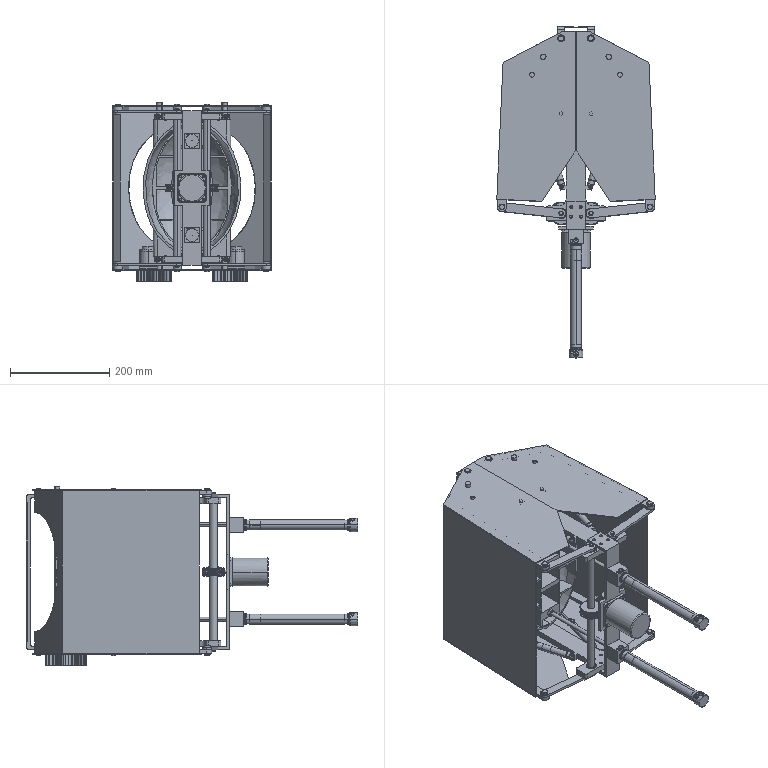Part | SolidWorks | features CompositeCurve 13, ReferencePattern 9, MirrorCompFeat 4 | 208 solids | 3784 faces | volume 3212108 mm3 | cylinder 1335 | plane 878 | spline 588 | cone 501 | torus 290 | sphere 192 | commonest cylinder face diameters 45.739 x128 10 x106 6 x104 12 x82 36.25 x68 47.5 x68